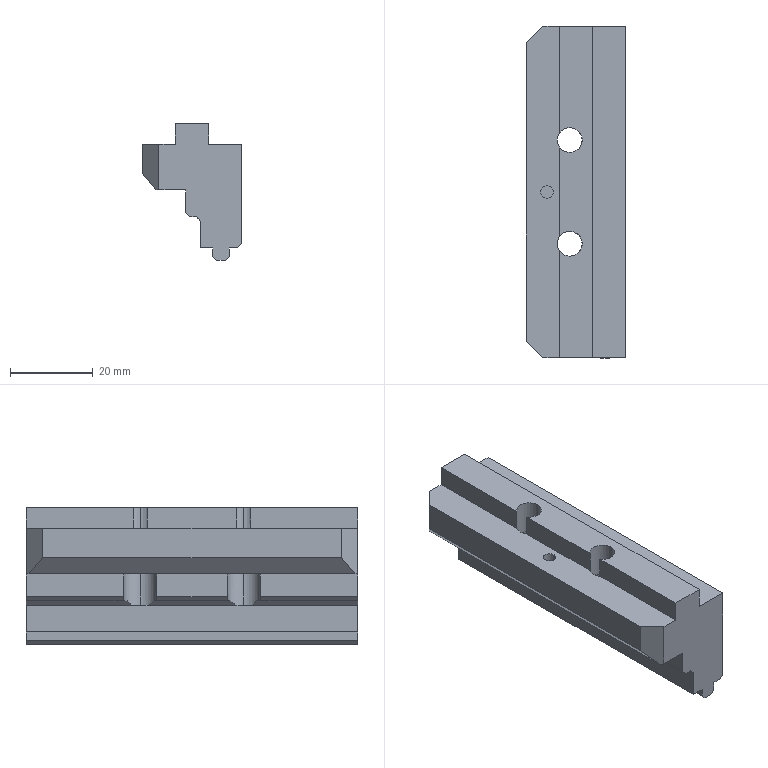Part | SolidWorks | features ICE 4, Chamfer 2, Extrusion 1 | 1 solid | 51 faces | box 24 x 80 x 33 mm | volume 35961 mm3 | plane 41 | cylinder 10 | commonest cylinder face diameters 6 x4 8 x4 3 x2